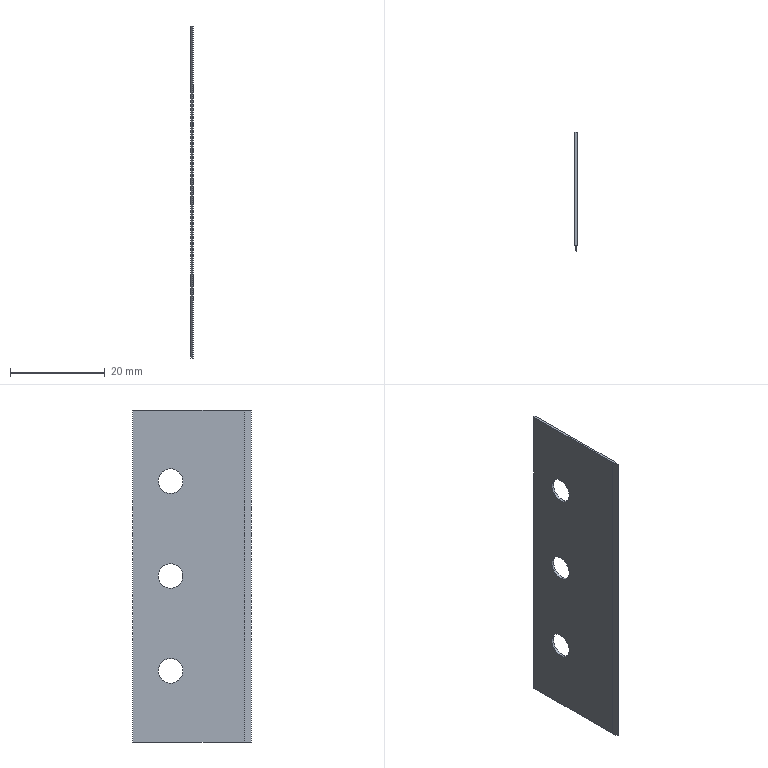Part | SolidWorks | features Extrusion 1, HoleWzd 1, ICE 1 | 1 solid | 13 faces | box 0.5 x 25 x 70 mm | volume 816.894 mm3 | plane 7 | cylinder 6 | commonest cylinder face diameters 5.2 x6
STEP:
#1=CARTESIAN_POINT('',(0.5,4.5,-17.4));
#2=VERTEX_POINT('',#1);
#3=CARTESIAN_POINT('',(0.5,4.5,-22.6));
#4=VERTEX_POINT('',#3);
#5=CARTESIAN_POINT('',(0.5,4.5,-20.));
#6=DIRECTION('',(1.,0.,0.));
#7=DIRECTION('',(0.,0.,-1.));
#8=AXIS2_PLACEMENT_3D('',#5,#6,#7);
#9=CIRCLE('',#8,2.6);
#10=EDGE_CURVE('',#2,#4,#9,.T.);
#11=ORIENTED_EDGE('',*,*,#10,.T.);
#12=CARTESIAN_POINT('',(0.,4.5,-22.6));
#13=VERTEX_POINT('',#12);
#14=CARTESIAN_POINT('',(0.,4.5,-22.6));
#15=DIRECTION('',(-1.,0.,0.));
#16=VECTOR('',#15,1000.);
#17=LINE('',#14,#16);
#18=EDGE_CURVE('',#4,#13,#17,.T.);
#19=ORIENTED_EDGE('',*,*,#18,.T.);
#20=CARTESIAN_POINT('',(0.,4.5,-17.4));
#21=VERTEX_POINT('',#20);
#22=CARTESIAN_POINT('',(0.,4.5,-20.));
#23=DIRECTION('',(-1.,0.,0.));
#24=DIRECTION('',(0.,0.,1.));
#25=AXIS2_PLACEMENT_3D('',#22,#23,#24);
#26=CIRCLE('',#25,2.6);
#27=EDGE_CURVE('',#13,#21,#26,.T.);
#28=ORIENTED_EDGE('',*,*,#27,.T.);
#29=CARTESIAN_POINT('',(0.,4.5,-17.4));
#30=DIRECTION('',(-1.,0.,0.));
#31=VECTOR('',#30,1000.);
#32=LINE('',#29,#31);
#33=EDGE_CURVE('',#2,#21,#32,.T.);
#34=ORIENTED_EDGE('',*,*,#33,.F.);
#35=EDGE_LOOP('',(#11,#19,#28,#34));
#36=FACE_OUTER_BOUND('',#35,.T.);
#37=CARTESIAN_POINT('',(0.,4.5,-20.));
#38=DIRECTION('',(-1.,0.,0.));
#39=DIRECTION('',(0.,0.,1.));
#40=AXIS2_PLACEMENT_3D('',#37,#38,#39);
#41=CYLINDRICAL_SURFACE('',#40,2.6);
#42=ADVANCED_FACE('',(#36),#41,.F.);
#43=CARTESIAN_POINT('',(0.5,4.5,2.6));
#44=VERTEX_POINT('',#43);
#45=CARTESIAN_POINT('',(0.5,4.5,-2.6));
#46=VERTEX_POINT('',#45);
#47=CARTESIAN_POINT('',(0.5,4.5,0.));
#48=DIRECTION('',(1.,0.,0.));
#49=DIRECTION('',(0.,0.,-1.));
#50=AXIS2_PLACEMENT_3D('',#47,#48,#49);
#51=CIRCLE('',#50,2.6);
#52=EDGE_CURVE('',#44,#46,#51,.T.);
#53=ORIENTED_EDGE('',*,*,#52,.T.);
#54=CARTESIAN_POINT('',(0.,4.5,-2.6));
#55=VERTEX_POINT('',#54);
#56=CARTESIAN_POINT('',(0.,4.5,-2.6));
#57=DIRECTION('',(-1.,0.,0.));
#58=VECTOR('',#57,1000.);
#59=LINE('',#56,#58);
#60=EDGE_CURVE('',#46,#55,#59,.T.);
#61=ORIENTED_EDGE('',*,*,#60,.T.);
#62=CARTESIAN_POINT('',(0.,4.5,2.6));
#63=VERTEX_POINT('',#62);
#64=CARTESIAN_POINT('',(0.,4.5,0.));
#65=DIRECTION('',(-1.,0.,0.));
#66=DIRECTION('',(0.,0.,1.));
#67=AXIS2_PLACEMENT_3D('',#64,#65,#66);
#68=CIRCLE('',#67,2.6);
#69=EDGE_CURVE('',#55,#63,#68,.T.);
#70=ORIENTED_EDGE('',*,*,#69,.T.);
#71=CARTESIAN_POINT('',(0.,4.5,2.6));
#72=DIRECTION('',(-1.,0.,0.));
#73=VECTOR('',#72,1000.);
#74=LINE('',#71,#73);
#75=EDGE_CURVE('',#44,#63,#74,.T.);
#76=ORIENTED_EDGE('',*,*,#75,.F.);
#77=EDGE_LOOP('',(#53,#61,#70,#76));
#78=FACE_OUTER_BOUND('',#77,.T.);
#79=CARTESIAN_POINT('',(0.,4.5,0.));
#80=DIRECTION('',(-1.,0.,0.));
#81=DIRECTION('',(0.,0.,1.));
#82=AXIS2_PLACEMENT_3D('',#79,#80,#81);
#83=CYLINDRICAL_SURFACE('',#82,2.6);
#84=ADVANCED_FACE('',(#78),#83,.F.);
#85=CARTESIAN_POINT('',(0.5,4.5,22.6));
#86=VERTEX_POINT('',#85);
#87=CARTESIAN_POINT('',(0.5,4.5,17.4));
#88=VERTEX_POINT('',#87);
#89=CARTESIAN_POINT('',(0.5,4.5,20.));
#90=DIRECTION('',(1.,0.,0.));
#91=DIRECTION('',(0.,0.,-1.));
#92=AXIS2_PLACEMENT_3D('',#89,#90,#91);
#93=CIRCLE('',#92,2.6);
#94=EDGE_CURVE('',#86,#88,#93,.T.);
#95=ORIENTED_EDGE('',*,*,#94,.T.);
#96=CARTESIAN_POINT('',(0.,4.5,17.4));
#97=VERTEX_POINT('',#96);
#98=CARTESIAN_POINT('',(0.,4.5,17.4));
#99=DIRECTION('',(-1.,0.,0.));
#100=VECTOR('',#99,1000.);
#101=LINE('',#98,#100);
#102=EDGE_CURVE('',#88,#97,#101,.T.);
#103=ORIENTED_EDGE('',*,*,#102,.T.);
#104=CARTESIAN_POINT('',(0.,4.5,22.6));
#105=VERTEX_POINT('',#104);
#106=CARTESIAN_POINT('',(0.,4.5,20.));
#107=DIRECTION('',(-1.,0.,0.));
#108=DIRECTION('',(0.,0.,1.));
#109=AXIS2_PLACEMENT_3D('',#106,#107,#108);
#110=CIRCLE('',#109,2.6);
#111=EDGE_CURVE('',#97,#105,#110,.T.);
#112=ORIENTED_EDGE('',*,*,#111,.T.);
#113=CARTESIAN_POINT('',(0.,4.5,22.6));
#114=DIRECTION('',(-1.,0.,0.));
#115=VECTOR('',#114,1000.);
#116=LINE('',#113,#115);
#117=EDGE_CURVE('',#86,#105,#116,.T.);
#118=ORIENTED_EDGE('',*,*,#117,.F.);
#119=EDGE_LOOP('',(#95,#103,#112,#118));
#120=FACE_OUTER_BOUND('',#119,.T.);
#121=CARTESIAN_POINT('',(0.,4.5,20.));
#122=DIRECTION('',(-1.,0.,0.));
#123=DIRECTION('',(0.,0.,1.));
#124=AXIS2_PLACEMENT_3D('',#121,#122,#123);
#125=CYLINDRICAL_SURFACE('',#124,2.6);
#126=ADVANCED_FACE('',(#120),#125,.F.);
#127=CARTESIAN_POINT('',(0.5,-11.,-35.));
#128=VERTEX_POINT('',#127);
#129=CARTESIAN_POINT('',(0.5,12.5,-35.));
#130=VERTEX_POINT('',#129);
#131=CARTESIAN_POINT('',(0.5,12.5,-35.));
#132=DIRECTION('',(0.,1.,0.));
#133=VECTOR('',#132,1000.);
#134=LINE('',#131,#133);
#135=EDGE_CURVE('',#128,#130,#134,.T.);
#136=ORIENTED_EDGE('',*,*,#135,.F.);
#137=CARTESIAN_POINT('',(0.25,-12.5,-35.));
#138=VERTEX_POINT('',#137);
#139=CARTESIAN_POINT('',(0.25,-12.5,-35.));
#140=DIRECTION('',(-0.1644,-0.9864,0.));
#141=VECTOR('',#140,1000.);
#142=LINE('',#139,#141);
#143=EDGE_CURVE('',#128,#138,#142,.T.);
#144=ORIENTED_EDGE('',*,*,#143,.T.);
#145=CARTESIAN_POINT('',(0.,-11.,-35.));
#146=VERTEX_POINT('',#145);
#147=CARTESIAN_POINT('',(0.25,-12.5,-35.));
#148=DIRECTION('',(-0.1644,0.9864,0.));
#149=VECTOR('',#148,1000.);
#150=LINE('',#147,#149);
#151=EDGE_CURVE('',#138,#146,#150,.T.);
#152=ORIENTED_EDGE('',*,*,#151,.T.);
#153=CARTESIAN_POINT('',(0.,12.5,-35.));
#154=VERTEX_POINT('',#153);
#155=CARTESIAN_POINT('',(0.,12.5,-35.));
#156=DIRECTION('',(0.,1.,0.));
#157=VECTOR('',#156,1000.);
#158=LINE('',#155,#157);
#159=EDGE_CURVE('',#146,#154,#158,.T.);
#160=ORIENTED_EDGE('',*,*,#159,.T.);
#161=CARTESIAN_POINT('',(0.5,12.5,-35.));
#162=DIRECTION('',(-1.,0.,0.));
#163=VECTOR('',#162,1000.);
#164=LINE('',#161,#163);
#165=EDGE_CURVE('',#130,#154,#164,.T.);
#166=ORIENTED_EDGE('',*,*,#165,.F.);
#167=EDGE_LOOP('',(#136,#144,#152,#160,#166));
#168=FACE_OUTER_BOUND('',#167,.T.);
#169=CARTESIAN_POINT('',(0.5,12.5,-35.));
#170=DIRECTION('',(0.,0.,1.));
#171=DIRECTION('',(1.,0.,0.));
#172=AXIS2_PLACEMENT_3D('',#169,#170,#171);
#173=PLANE('',#172);
#174=ADVANCED_FACE('',(#168),#173,.F.);
#175=CARTESIAN_POINT('',(0.,12.5,35.));
#176=VERTEX_POINT('',#175);
#177=CARTESIAN_POINT('',(0.,12.5,35.));
#178=DIRECTION('',(0.,0.,1.));
#179=VECTOR('',#178,1000.);
#180=LINE('',#177,#179);
#181=EDGE_CURVE('',#154,#176,#180,.T.);
#182=ORIENTED_EDGE('',*,*,#181,.T.);
#183=CARTESIAN_POINT('',(0.5,12.5,35.));
#184=VERTEX_POINT('',#183);
#185=CARTESIAN_POINT('',(0.5,12.5,35.));
#186=DIRECTION('',(-1.,0.,0.));
#187=VECTOR('',#186,1000.);
#188=LINE('',#185,#187);
#189=EDGE_CURVE('',#184,#176,#188,.T.);
#190=ORIENTED_EDGE('',*,*,#189,.F.);
#191=CARTESIAN_POINT('',(0.5,12.5,35.));
#192=DIRECTION('',(0.,0.,1.));
#193=VECTOR('',#192,1000.);
#194=LINE('',#191,#193);
#195=EDGE_CURVE('',#130,#184,#194,.T.);
#196=ORIENTED_EDGE('',*,*,#195,.F.);
#197=ORIENTED_EDGE('',*,*,#165,.T.);
#198=EDGE_LOOP('',(#182,#190,#196,#197));
#199=FACE_OUTER_BOUND('',#198,.T.);
#200=CARTESIAN_POINT('',(0.5,12.5,35.));
#201=DIRECTION('',(0.,-1.,0.));
#202=DIRECTION('',(0.,0.,-1.));
#203=AXIS2_PLACEMENT_3D('',#200,#201,#202);
#204=PLANE('',#203);
#205=ADVANCED_FACE('',(#199),#204,.F.);
#206=CARTESIAN_POINT('',(0.25,-12.5,35.));
#207=VERTEX_POINT('',#206);
#208=CARTESIAN_POINT('',(0.,-11.,35.));
#209=VERTEX_POINT('',#208);
#210=CARTESIAN_POINT('',(0.25,-12.5,35.));
#211=DIRECTION('',(-0.1644,0.9864,0.));
#212=VECTOR('',#211,1000.);
#213=LINE('',#210,#212);
#214=EDGE_CURVE('',#207,#209,#213,.T.);
#215=ORIENTED_EDGE('',*,*,#214,.F.);
#216=CARTESIAN_POINT('',(0.5,-11.,35.));
#217=VERTEX_POINT('',#216);
#218=CARTESIAN_POINT('',(0.25,-12.5,35.));
#219=DIRECTION('',(-0.1644,-0.9864,0.));
#220=VECTOR('',#219,1000.);
#221=LINE('',#218,#220);
#222=EDGE_CURVE('',#217,#207,#221,.T.);
#223=ORIENTED_EDGE('',*,*,#222,.F.);
#224=CARTESIAN_POINT('',(0.5,12.5,35.));
#225=DIRECTION('',(0.,-1.,0.));
#226=VECTOR('',#225,1000.);
#227=LINE('',#224,#226);
#228=EDGE_CURVE('',#184,#217,#227,.T.);
#229=ORIENTED_EDGE('',*,*,#228,.F.);
#230=ORIENTED_EDGE('',*,*,#189,.T.);
#231=CARTESIAN_POINT('',(0.,12.5,35.));
#232=DIRECTION('',(0.,-1.,0.));
#233=VECTOR('',#232,1000.);
#234=LINE('',#231,#233);
#235=EDGE_CURVE('',#176,#209,#234,.T.);
#236=ORIENTED_EDGE('',*,*,#235,.T.);
#237=EDGE_LOOP('',(#215,#223,#229,#230,#236));
#238=FACE_OUTER_BOUND('',#237,.T.);
#239=CARTESIAN_POINT('',(0.5,12.5,35.));
#240=DIRECTION('',(0.,0.,-1.));
#241=DIRECTION('',(0.,1.,0.));
#242=AXIS2_PLACEMENT_3D('',#239,#240,#241);
#243=PLANE('',#242);
#244=ADVANCED_FACE('',(#238),#243,.F.);
#245=ORIENTED_EDGE('',*,*,#10,.F.);
#246=CARTESIAN_POINT('',(0.5,4.5,-20.));
#247=DIRECTION('',(1.,0.,0.));
#248=DIRECTION('',(0.,0.,-1.));
#249=AXIS2_PLACEMENT_3D('',#246,#247,#248);
#250=CIRCLE('',#249,2.6);
#251=EDGE_CURVE('',#4,#2,#250,.T.);
#252=ORIENTED_EDGE('',*,*,#251,.F.);
#253=EDGE_LOOP('',(#245,#252));
#254=FACE_BOUND('',#253,.T.);
#255=ORIENTED_EDGE('',*,*,#52,.F.);
#256=CARTESIAN_POINT('',(0.5,4.5,0.));
#257=DIRECTION('',(1.,0.,0.));
#258=DIRECTION('',(0.,0.,-1.));
#259=AXIS2_PLACEMENT_3D('',#256,#257,#258);
#260=CIRCLE('',#259,2.6);
#261=EDGE_CURVE('',#46,#44,#260,.T.);
#262=ORIENTED_EDGE('',*,*,#261,.F.);
#263=EDGE_LOOP('',(#255,#262));
#264=FACE_BOUND('',#263,.T.);
#265=ORIENTED_EDGE('',*,*,#94,.F.);
#266=CARTESIAN_POINT('',(0.5,4.5,20.));
#267=DIRECTION('',(1.,0.,0.));
#268=DIRECTION('',(0.,0.,-1.));
#269=AXIS2_PLACEMENT_3D('',#266,#267,#268);
#270=CIRCLE('',#269,2.6);
#271=EDGE_CURVE('',#88,#86,#270,.T.);
#272=ORIENTED_EDGE('',*,*,#271,.F.);
#273=EDGE_LOOP('',(#265,#272));
#274=FACE_BOUND('',#273,.T.);
#275=CARTESIAN_POINT('',(0.5,-11.,-35.));
#276=DIRECTION('',(0.,0.,1.));
#277=VECTOR('',#276,1000.);
#278=LINE('',#275,#277);
#279=EDGE_CURVE('',#128,#217,#278,.T.);
#280=ORIENTED_EDGE('',*,*,#279,.F.);
#281=ORIENTED_EDGE('',*,*,#135,.T.);
#282=ORIENTED_EDGE('',*,*,#195,.T.);
#283=ORIENTED_EDGE('',*,*,#228,.T.);
#284=EDGE_LOOP('',(#280,#281,#282,#283));
#285=FACE_OUTER_BOUND('',#284,.T.);
#286=CARTESIAN_POINT('',(0.5,0.,0.));
#287=DIRECTION('',(1.,0.,0.));
#288=DIRECTION('',(0.,0.,-1.));
#289=AXIS2_PLACEMENT_3D('',#286,#287,#288);
#290=PLANE('',#289);
#291=ADVANCED_FACE('',(#254,#264,#274,#285),#290,.T.);
#292=CARTESIAN_POINT('',(0.,4.5,-20.));
#293=DIRECTION('',(-1.,0.,0.));
#294=DIRECTION('',(0.,0.,1.));
#295=AXIS2_PLACEMENT_3D('',#292,#293,#294);
#296=CIRCLE('',#295,2.6);
#297=EDGE_CURVE('',#21,#13,#296,.T.);
#298=ORIENTED_EDGE('',*,*,#297,.F.);
#299=ORIENTED_EDGE('',*,*,#27,.F.);
#300=EDGE_LOOP('',(#298,#299));
#301=FACE_BOUND('',#300,.T.);
#302=CARTESIAN_POINT('',(0.,4.5,0.));
#303=DIRECTION('',(-1.,0.,0.));
#304=DIRECTION('',(0.,0.,1.));
#305=AXIS2_PLACEMENT_3D('',#302,#303,#304);
#306=CIRCLE('',#305,2.6);
#307=EDGE_CURVE('',#63,#55,#306,.T.);
#308=ORIENTED_EDGE('',*,*,#307,.F.);
#309=ORIENTED_EDGE('',*,*,#69,.F.);
#310=EDGE_LOOP('',(#308,#309));
#311=FACE_BOUND('',#310,.T.);
#312=CARTESIAN_POINT('',(0.,4.5,20.));
#313=DIRECTION('',(-1.,0.,0.));
#314=DIRECTION('',(0.,0.,1.));
#315=AXIS2_PLACEMENT_3D('',#312,#313,#314);
#316=CIRCLE('',#315,2.6);
#317=EDGE_CURVE('',#105,#97,#316,.T.);
#318=ORIENTED_EDGE('',*,*,#317,.F.);
#319=ORIENTED_EDGE('',*,*,#111,.F.);
#320=EDGE_LOOP('',(#318,#319));
#321=FACE_BOUND('',#320,.T.);
#322=ORIENTED_EDGE('',*,*,#159,.F.);
#323=CARTESIAN_POINT('',(0.,-11.,-35.));
#324=DIRECTION('',(0.,0.,1.));
#325=VECTOR('',#324,1000.);
#326=LINE('',#323,#325);
#327=EDGE_CURVE('',#146,#209,#326,.T.);
#328=ORIENTED_EDGE('',*,*,#327,.T.);
#329=ORIENTED_EDGE('',*,*,#235,.F.);
#330=ORIENTED_EDGE('',*,*,#181,.F.);
#331=EDGE_LOOP('',(#322,#328,#329,#330));
#332=FACE_OUTER_BOUND('',#331,.T.);
#333=CARTESIAN_POINT('',(0.,0.,0.));
#334=DIRECTION('',(1.,0.,0.));
#335=DIRECTION('',(0.,0.,-1.));
#336=AXIS2_PLACEMENT_3D('',#333,#334,#335);
#337=PLANE('',#336);
#338=ADVANCED_FACE('',(#301,#311,#321,#332),#337,.F.);
#339=ORIENTED_EDGE('',*,*,#222,.T.);
#340=CARTESIAN_POINT('',(0.25,-12.5,-35.));
#341=DIRECTION('',(0.,0.,1.));
#342=VECTOR('',#341,1000.);
#343=LINE('',#340,#342);
#344=EDGE_CURVE('',#138,#207,#343,.T.);
#345=ORIENTED_EDGE('',*,*,#344,.F.);
#346=ORIENTED_EDGE('',*,*,#143,.F.);
#347=ORIENTED_EDGE('',*,*,#279,.T.);
#348=EDGE_LOOP('',(#339,#345,#346,#347));
#349=FACE_OUTER_BOUND('',#348,.T.);
#350=CARTESIAN_POINT('',(0.25,-12.5,-35.));
#351=DIRECTION('',(-0.9864,0.1644,0.));
#352=DIRECTION('',(-0.1644,-0.9864,0.));
#353=AXIS2_PLACEMENT_3D('',#350,#351,#352);
#354=PLANE('',#353);
#355=ADVANCED_FACE('',(#349),#354,.F.);
#356=ORIENTED_EDGE('',*,*,#214,.T.);
#357=ORIENTED_EDGE('',*,*,#327,.F.);
#358=ORIENTED_EDGE('',*,*,#151,.F.);
#359=ORIENTED_EDGE('',*,*,#344,.T.);
#360=EDGE_LOOP('',(#356,#357,#358,#359));
#361=FACE_OUTER_BOUND('',#360,.T.);
#362=CARTESIAN_POINT('',(0.25,-12.5,-35.));
#363=DIRECTION('',(0.9864,0.1644,0.));
#364=DIRECTION('',(-0.1644,0.9864,0.));
#365=AXIS2_PLACEMENT_3D('',#362,#363,#364);
#366=PLANE('',#365);
#367=ADVANCED_FACE('',(#361),#366,.F.);
#368=ORIENTED_EDGE('',*,*,#102,.F.);
#369=ORIENTED_EDGE('',*,*,#271,.T.);
#370=ORIENTED_EDGE('',*,*,#117,.T.);
#371=ORIENTED_EDGE('',*,*,#317,.T.);
#372=EDGE_LOOP('',(#368,#369,#370,#371));
#373=FACE_OUTER_BOUND('',#372,.T.);
#374=CARTESIAN_POINT('',(0.,4.5,20.));
#375=DIRECTION('',(-1.,0.,0.));
#376=DIRECTION('',(0.,0.,1.));
#377=AXIS2_PLACEMENT_3D('',#374,#375,#376);
#378=CYLINDRICAL_SURFACE('',#377,2.6);
#379=ADVANCED_FACE('',(#373),#378,.F.);
#380=ORIENTED_EDGE('',*,*,#60,.F.);
#381=ORIENTED_EDGE('',*,*,#261,.T.);
#382=ORIENTED_EDGE('',*,*,#75,.T.);
#383=ORIENTED_EDGE('',*,*,#307,.T.);
#384=EDGE_LOOP('',(#380,#381,#382,#383));
#385=FACE_OUTER_BOUND('',#384,.T.);
#386=CARTESIAN_POINT('',(0.,4.5,0.));
#387=DIRECTION('',(-1.,0.,0.));
#388=DIRECTION('',(0.,0.,1.));
#389=AXIS2_PLACEMENT_3D('',#386,#387,#388);
#390=CYLINDRICAL_SURFACE('',#389,2.6);
#391=ADVANCED_FACE('',(#385),#390,.F.);
#392=ORIENTED_EDGE('',*,*,#18,.F.);
#393=ORIENTED_EDGE('',*,*,#251,.T.);
#394=ORIENTED_EDGE('',*,*,#33,.T.);
#395=ORIENTED_EDGE('',*,*,#297,.T.);
#396=EDGE_LOOP('',(#392,#393,#394,#395));
#397=FACE_OUTER_BOUND('',#396,.T.);
#398=CARTESIAN_POINT('',(0.,4.5,-20.));
#399=DIRECTION('',(-1.,0.,0.));
#400=DIRECTION('',(0.,0.,1.));
#401=AXIS2_PLACEMENT_3D('',#398,#399,#400);
#402=CYLINDRICAL_SURFACE('',#401,2.6);
#403=ADVANCED_FACE('',(#397),#402,.F.);
#404=CLOSED_SHELL('',(#42,#84,#126,#174,#205,#244,#291,#338,#355,#367,#379,#391,#403));
#405=MANIFOLD_SOLID_BREP('',#404);
#406=CARTESIAN_POINT('',(0.,0.,0.));
#407=DIRECTION('',(0.,0.,1.));
#408=DIRECTION('',(1.,0.,0.));
#409=AXIS2_PLACEMENT_3D('',#406,#407,#408);
#410=(LENGTH_UNIT()NAMED_UNIT(*)SI_UNIT(.MILLI.,.METRE.));
#411=UNCERTAINTY_MEASURE_WITH_UNIT(LENGTH_MEASURE(0.00001),#410,'','');
#412=(NAMED_UNIT(*)PLANE_ANGLE_UNIT()SI_UNIT($,.RADIAN.));
#413=(NAMED_UNIT(*)SI_UNIT($,.STERADIAN.)SOLID_ANGLE_UNIT());
#414=(GEOMETRIC_REPRESENTATION_CONTEXT(3)GLOBAL_UNCERTAINTY_ASSIGNED_CONTEXT((#411))GLOBAL_UNIT_ASSIGNED_CONTEXT((#410,#412,#413))REPRESENTATION_CONTEXT('',''));
#415=ADVANCED_BREP_SHAPE_REPRESENTATION('',(#405,#409),#414);